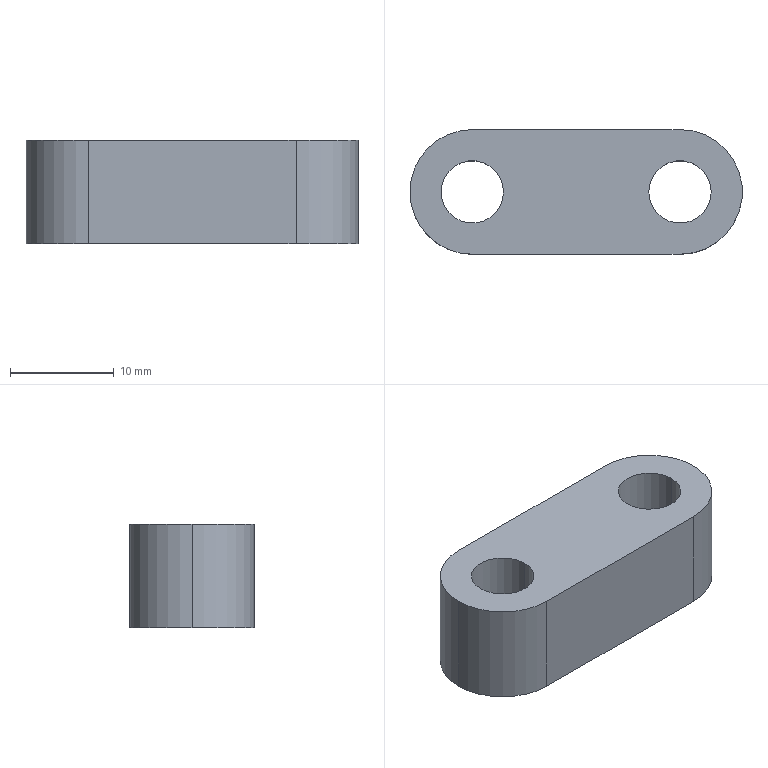Part | SolidWorks | features Extrusion 1 | 1 solid | 11 faces | box 32 x 12 x 10 mm | volume 2965 mm3 | cylinder 7 | plane 4 | commonest cylinder face diameters 6 x4 12 x3
STEP:
#1=CARTESIAN_POINT('',(17.,0.,10.));
#2=VERTEX_POINT('',#1);
#3=CARTESIAN_POINT('',(23.,0.,10.));
#4=VERTEX_POINT('',#3);
#5=CARTESIAN_POINT('',(20.,0.,10.));
#6=DIRECTION('',(0.,0.,1.));
#7=DIRECTION('',(1.,0.,0.));
#8=AXIS2_PLACEMENT_3D('',#5,#6,#7);
#9=CIRCLE('',#8,3.);
#10=EDGE_CURVE('',#2,#4,#9,.T.);
#11=ORIENTED_EDGE('',*,*,#10,.T.);
#12=CARTESIAN_POINT('',(23.,0.,0.));
#13=VERTEX_POINT('',#12);
#14=CARTESIAN_POINT('',(23.,0.,10.));
#15=DIRECTION('',(0.,0.,-1.));
#16=VECTOR('',#15,1000.);
#17=LINE('',#14,#16);
#18=EDGE_CURVE('',#4,#13,#17,.T.);
#19=ORIENTED_EDGE('',*,*,#18,.T.);
#20=CARTESIAN_POINT('',(17.,0.,0.));
#21=VERTEX_POINT('',#20);
#22=CARTESIAN_POINT('',(20.,0.,0.));
#23=DIRECTION('',(0.,0.,1.));
#24=DIRECTION('',(1.,0.,0.));
#25=AXIS2_PLACEMENT_3D('',#22,#23,#24);
#26=CIRCLE('',#25,3.);
#27=EDGE_CURVE('',#21,#13,#26,.T.);
#28=ORIENTED_EDGE('',*,*,#27,.F.);
#29=CARTESIAN_POINT('',(17.,0.,10.));
#30=DIRECTION('',(0.,0.,-1.));
#31=VECTOR('',#30,1000.);
#32=LINE('',#29,#31);
#33=EDGE_CURVE('',#2,#21,#32,.T.);
#34=ORIENTED_EDGE('',*,*,#33,.F.);
#35=EDGE_LOOP('',(#11,#19,#28,#34));
#36=FACE_OUTER_BOUND('',#35,.T.);
#37=CARTESIAN_POINT('',(20.,0.,10.));
#38=DIRECTION('',(0.,0.,-1.));
#39=DIRECTION('',(-1.,0.,0.));
#40=AXIS2_PLACEMENT_3D('',#37,#38,#39);
#41=CYLINDRICAL_SURFACE('',#40,3.);
#42=ADVANCED_FACE('',(#36),#41,.F.);
#43=CARTESIAN_POINT('',(-3.,0.,10.));
#44=VERTEX_POINT('',#43);
#45=CARTESIAN_POINT('',(3.,0.,10.));
#46=VERTEX_POINT('',#45);
#47=CARTESIAN_POINT('',(0.,0.,10.));
#48=DIRECTION('',(0.,0.,1.));
#49=DIRECTION('',(1.,0.,0.));
#50=AXIS2_PLACEMENT_3D('',#47,#48,#49);
#51=CIRCLE('',#50,3.);
#52=EDGE_CURVE('',#44,#46,#51,.T.);
#53=ORIENTED_EDGE('',*,*,#52,.T.);
#54=CARTESIAN_POINT('',(3.,0.,0.));
#55=VERTEX_POINT('',#54);
#56=CARTESIAN_POINT('',(3.,0.,10.));
#57=DIRECTION('',(0.,0.,-1.));
#58=VECTOR('',#57,1000.);
#59=LINE('',#56,#58);
#60=EDGE_CURVE('',#46,#55,#59,.T.);
#61=ORIENTED_EDGE('',*,*,#60,.T.);
#62=CARTESIAN_POINT('',(-3.,0.,0.));
#63=VERTEX_POINT('',#62);
#64=CARTESIAN_POINT('',(0.,0.,0.));
#65=DIRECTION('',(0.,0.,1.));
#66=DIRECTION('',(1.,0.,0.));
#67=AXIS2_PLACEMENT_3D('',#64,#65,#66);
#68=CIRCLE('',#67,3.);
#69=EDGE_CURVE('',#63,#55,#68,.T.);
#70=ORIENTED_EDGE('',*,*,#69,.F.);
#71=CARTESIAN_POINT('',(-3.,0.,10.));
#72=DIRECTION('',(0.,0.,-1.));
#73=VECTOR('',#72,1000.);
#74=LINE('',#71,#73);
#75=EDGE_CURVE('',#44,#63,#74,.T.);
#76=ORIENTED_EDGE('',*,*,#75,.F.);
#77=EDGE_LOOP('',(#53,#61,#70,#76));
#78=FACE_OUTER_BOUND('',#77,.T.);
#79=CARTESIAN_POINT('',(0.,0.,10.));
#80=DIRECTION('',(0.,0.,-1.));
#81=DIRECTION('',(-1.,0.,0.));
#82=AXIS2_PLACEMENT_3D('',#79,#80,#81);
#83=CYLINDRICAL_SURFACE('',#82,3.);
#84=ADVANCED_FACE('',(#78),#83,.F.);
#85=CARTESIAN_POINT('',(-6.,0.,10.));
#86=VERTEX_POINT('',#85);
#87=CARTESIAN_POINT('',(0.,-6.,10.));
#88=VERTEX_POINT('',#87);
#89=CARTESIAN_POINT('',(0.,0.,10.));
#90=DIRECTION('',(0.,0.,1.));
#91=DIRECTION('',(1.,0.,0.));
#92=AXIS2_PLACEMENT_3D('',#89,#90,#91);
#93=CIRCLE('',#92,6.);
#94=EDGE_CURVE('',#86,#88,#93,.T.);
#95=ORIENTED_EDGE('',*,*,#94,.F.);
#96=CARTESIAN_POINT('',(-6.,0.,0.));
#97=VERTEX_POINT('',#96);
#98=CARTESIAN_POINT('',(-6.,0.,10.));
#99=DIRECTION('',(0.,0.,-1.));
#100=VECTOR('',#99,1000.);
#101=LINE('',#98,#100);
#102=EDGE_CURVE('',#86,#97,#101,.T.);
#103=ORIENTED_EDGE('',*,*,#102,.T.);
#104=CARTESIAN_POINT('',(0.,-6.,0.));
#105=VERTEX_POINT('',#104);
#106=CARTESIAN_POINT('',(0.,0.,0.));
#107=DIRECTION('',(0.,0.,1.));
#108=DIRECTION('',(1.,0.,0.));
#109=AXIS2_PLACEMENT_3D('',#106,#107,#108);
#110=CIRCLE('',#109,6.);
#111=EDGE_CURVE('',#97,#105,#110,.T.);
#112=ORIENTED_EDGE('',*,*,#111,.T.);
#113=CARTESIAN_POINT('',(0.,-6.,10.));
#114=DIRECTION('',(0.,0.,-1.));
#115=VECTOR('',#114,1000.);
#116=LINE('',#113,#115);
#117=EDGE_CURVE('',#88,#105,#116,.T.);
#118=ORIENTED_EDGE('',*,*,#117,.F.);
#119=EDGE_LOOP('',(#95,#103,#112,#118));
#120=FACE_OUTER_BOUND('',#119,.T.);
#121=CARTESIAN_POINT('',(0.,0.,10.));
#122=DIRECTION('',(0.,0.,-1.));
#123=DIRECTION('',(-1.,0.,0.));
#124=AXIS2_PLACEMENT_3D('',#121,#122,#123);
#125=CYLINDRICAL_SURFACE('',#124,6.);
#126=ADVANCED_FACE('',(#120),#125,.T.);
#127=ORIENTED_EDGE('',*,*,#52,.F.);
#128=CARTESIAN_POINT('',(0.,0.,10.));
#129=DIRECTION('',(0.,0.,1.));
#130=DIRECTION('',(1.,0.,0.));
#131=AXIS2_PLACEMENT_3D('',#128,#129,#130);
#132=CIRCLE('',#131,3.);
#133=EDGE_CURVE('',#46,#44,#132,.T.);
#134=ORIENTED_EDGE('',*,*,#133,.F.);
#135=EDGE_LOOP('',(#127,#134));
#136=FACE_BOUND('',#135,.T.);
#137=CARTESIAN_POINT('',(0.,6.,10.));
#138=VERTEX_POINT('',#137);
#139=CARTESIAN_POINT('',(0.,0.,10.));
#140=DIRECTION('',(0.,0.,1.));
#141=DIRECTION('',(1.,0.,0.));
#142=AXIS2_PLACEMENT_3D('',#139,#140,#141);
#143=CIRCLE('',#142,6.);
#144=EDGE_CURVE('',#138,#86,#143,.T.);
#145=ORIENTED_EDGE('',*,*,#144,.T.);
#146=ORIENTED_EDGE('',*,*,#94,.T.);
#147=CARTESIAN_POINT('',(20.,-6.,10.));
#148=VERTEX_POINT('',#147);
#149=CARTESIAN_POINT('',(0.,-6.,10.));
#150=DIRECTION('',(1.,0.,0.));
#151=VECTOR('',#150,1000.);
#152=LINE('',#149,#151);
#153=EDGE_CURVE('',#88,#148,#152,.T.);
#154=ORIENTED_EDGE('',*,*,#153,.T.);
#155=CARTESIAN_POINT('',(20.,6.,10.));
#156=VERTEX_POINT('',#155);
#157=CARTESIAN_POINT('',(20.,0.,10.));
#158=DIRECTION('',(0.,0.,1.));
#159=DIRECTION('',(1.,0.,0.));
#160=AXIS2_PLACEMENT_3D('',#157,#158,#159);
#161=CIRCLE('',#160,6.);
#162=EDGE_CURVE('',#148,#156,#161,.T.);
#163=ORIENTED_EDGE('',*,*,#162,.T.);
#164=CARTESIAN_POINT('',(0.,6.,10.));
#165=DIRECTION('',(-1.,0.,0.));
#166=VECTOR('',#165,1000.);
#167=LINE('',#164,#166);
#168=EDGE_CURVE('',#156,#138,#167,.T.);
#169=ORIENTED_EDGE('',*,*,#168,.T.);
#170=EDGE_LOOP('',(#145,#146,#154,#163,#169));
#171=FACE_OUTER_BOUND('',#170,.T.);
#172=ORIENTED_EDGE('',*,*,#10,.F.);
#173=CARTESIAN_POINT('',(20.,0.,10.));
#174=DIRECTION('',(0.,0.,1.));
#175=DIRECTION('',(1.,0.,0.));
#176=AXIS2_PLACEMENT_3D('',#173,#174,#175);
#177=CIRCLE('',#176,3.);
#178=EDGE_CURVE('',#4,#2,#177,.T.);
#179=ORIENTED_EDGE('',*,*,#178,.F.);
#180=EDGE_LOOP('',(#172,#179));
#181=FACE_BOUND('',#180,.T.);
#182=CARTESIAN_POINT('',(0.,0.,10.));
#183=DIRECTION('',(0.,0.,1.));
#184=DIRECTION('',(1.,0.,0.));
#185=AXIS2_PLACEMENT_3D('',#182,#183,#184);
#186=PLANE('',#185);
#187=ADVANCED_FACE('',(#136,#171,#181),#186,.T.);
#188=CARTESIAN_POINT('',(0.,6.,0.));
#189=VERTEX_POINT('',#188);
#190=CARTESIAN_POINT('',(0.,0.,0.));
#191=DIRECTION('',(0.,0.,1.));
#192=DIRECTION('',(1.,0.,0.));
#193=AXIS2_PLACEMENT_3D('',#190,#191,#192);
#194=CIRCLE('',#193,6.);
#195=EDGE_CURVE('',#189,#97,#194,.T.);
#196=ORIENTED_EDGE('',*,*,#195,.F.);
#197=CARTESIAN_POINT('',(20.,6.,0.));
#198=VERTEX_POINT('',#197);
#199=CARTESIAN_POINT('',(0.,6.,0.));
#200=DIRECTION('',(-1.,0.,0.));
#201=VECTOR('',#200,1000.);
#202=LINE('',#199,#201);
#203=EDGE_CURVE('',#198,#189,#202,.T.);
#204=ORIENTED_EDGE('',*,*,#203,.F.);
#205=CARTESIAN_POINT('',(20.,-6.,0.));
#206=VERTEX_POINT('',#205);
#207=CARTESIAN_POINT('',(20.,0.,0.));
#208=DIRECTION('',(0.,0.,1.));
#209=DIRECTION('',(1.,0.,0.));
#210=AXIS2_PLACEMENT_3D('',#207,#208,#209);
#211=CIRCLE('',#210,6.);
#212=EDGE_CURVE('',#206,#198,#211,.T.);
#213=ORIENTED_EDGE('',*,*,#212,.F.);
#214=CARTESIAN_POINT('',(0.,-6.,0.));
#215=DIRECTION('',(1.,0.,0.));
#216=VECTOR('',#215,1000.);
#217=LINE('',#214,#216);
#218=EDGE_CURVE('',#105,#206,#217,.T.);
#219=ORIENTED_EDGE('',*,*,#218,.F.);
#220=ORIENTED_EDGE('',*,*,#111,.F.);
#221=EDGE_LOOP('',(#196,#204,#213,#219,#220));
#222=FACE_OUTER_BOUND('',#221,.T.);
#223=ORIENTED_EDGE('',*,*,#69,.T.);
#224=CARTESIAN_POINT('',(0.,0.,0.));
#225=DIRECTION('',(0.,0.,1.));
#226=DIRECTION('',(1.,0.,0.));
#227=AXIS2_PLACEMENT_3D('',#224,#225,#226);
#228=CIRCLE('',#227,3.);
#229=EDGE_CURVE('',#55,#63,#228,.T.);
#230=ORIENTED_EDGE('',*,*,#229,.T.);
#231=EDGE_LOOP('',(#223,#230));
#232=FACE_BOUND('',#231,.T.);
#233=ORIENTED_EDGE('',*,*,#27,.T.);
#234=CARTESIAN_POINT('',(20.,0.,0.));
#235=DIRECTION('',(0.,0.,1.));
#236=DIRECTION('',(1.,0.,0.));
#237=AXIS2_PLACEMENT_3D('',#234,#235,#236);
#238=CIRCLE('',#237,3.);
#239=EDGE_CURVE('',#13,#21,#238,.T.);
#240=ORIENTED_EDGE('',*,*,#239,.T.);
#241=EDGE_LOOP('',(#233,#240));
#242=FACE_BOUND('',#241,.T.);
#243=CARTESIAN_POINT('',(0.,0.,0.));
#244=DIRECTION('',(0.,0.,1.));
#245=DIRECTION('',(1.,0.,0.));
#246=AXIS2_PLACEMENT_3D('',#243,#244,#245);
#247=PLANE('',#246);
#248=ADVANCED_FACE('',(#222,#232,#242),#247,.F.);
#249=ORIENTED_EDGE('',*,*,#102,.F.);
#250=ORIENTED_EDGE('',*,*,#144,.F.);
#251=CARTESIAN_POINT('',(0.,6.,10.));
#252=DIRECTION('',(0.,0.,-1.));
#253=VECTOR('',#252,1000.);
#254=LINE('',#251,#253);
#255=EDGE_CURVE('',#138,#189,#254,.T.);
#256=ORIENTED_EDGE('',*,*,#255,.T.);
#257=ORIENTED_EDGE('',*,*,#195,.T.);
#258=EDGE_LOOP('',(#249,#250,#256,#257));
#259=FACE_OUTER_BOUND('',#258,.T.);
#260=CARTESIAN_POINT('',(0.,0.,10.));
#261=DIRECTION('',(0.,0.,-1.));
#262=DIRECTION('',(-1.,0.,0.));
#263=AXIS2_PLACEMENT_3D('',#260,#261,#262);
#264=CYLINDRICAL_SURFACE('',#263,6.);
#265=ADVANCED_FACE('',(#259),#264,.T.);
#266=ORIENTED_EDGE('',*,*,#218,.T.);
#267=CARTESIAN_POINT('',(20.,-6.,10.));
#268=DIRECTION('',(0.,0.,-1.));
#269=VECTOR('',#268,1000.);
#270=LINE('',#267,#269);
#271=EDGE_CURVE('',#148,#206,#270,.T.);
#272=ORIENTED_EDGE('',*,*,#271,.F.);
#273=ORIENTED_EDGE('',*,*,#153,.F.);
#274=ORIENTED_EDGE('',*,*,#117,.T.);
#275=EDGE_LOOP('',(#266,#272,#273,#274));
#276=FACE_OUTER_BOUND('',#275,.T.);
#277=CARTESIAN_POINT('',(0.,-6.,10.));
#278=DIRECTION('',(0.,1.,0.));
#279=DIRECTION('',(0.,0.,1.));
#280=AXIS2_PLACEMENT_3D('',#277,#278,#279);
#281=PLANE('',#280);
#282=ADVANCED_FACE('',(#276),#281,.F.);
#283=ORIENTED_EDGE('',*,*,#212,.T.);
#284=CARTESIAN_POINT('',(20.,6.,10.));
#285=DIRECTION('',(0.,0.,-1.));
#286=VECTOR('',#285,1000.);
#287=LINE('',#284,#286);
#288=EDGE_CURVE('',#156,#198,#287,.T.);
#289=ORIENTED_EDGE('',*,*,#288,.F.);
#290=ORIENTED_EDGE('',*,*,#162,.F.);
#291=ORIENTED_EDGE('',*,*,#271,.T.);
#292=EDGE_LOOP('',(#283,#289,#290,#291));
#293=FACE_OUTER_BOUND('',#292,.T.);
#294=CARTESIAN_POINT('',(20.,0.,10.));
#295=DIRECTION('',(0.,0.,-1.));
#296=DIRECTION('',(-1.,0.,0.));
#297=AXIS2_PLACEMENT_3D('',#294,#295,#296);
#298=CYLINDRICAL_SURFACE('',#297,6.);
#299=ADVANCED_FACE('',(#293),#298,.T.);
#300=ORIENTED_EDGE('',*,*,#203,.T.);
#301=ORIENTED_EDGE('',*,*,#255,.F.);
#302=ORIENTED_EDGE('',*,*,#168,.F.);
#303=ORIENTED_EDGE('',*,*,#288,.T.);
#304=EDGE_LOOP('',(#300,#301,#302,#303));
#305=FACE_OUTER_BOUND('',#304,.T.);
#306=CARTESIAN_POINT('',(0.,6.,10.));
#307=DIRECTION('',(0.,-1.,0.));
#308=DIRECTION('',(0.,0.,-1.));
#309=AXIS2_PLACEMENT_3D('',#306,#307,#308);
#310=PLANE('',#309);
#311=ADVANCED_FACE('',(#305),#310,.F.);
#312=ORIENTED_EDGE('',*,*,#60,.F.);
#313=ORIENTED_EDGE('',*,*,#133,.T.);
#314=ORIENTED_EDGE('',*,*,#75,.T.);
#315=ORIENTED_EDGE('',*,*,#229,.F.);
#316=EDGE_LOOP('',(#312,#313,#314,#315));
#317=FACE_OUTER_BOUND('',#316,.T.);
#318=CARTESIAN_POINT('',(0.,0.,10.));
#319=DIRECTION('',(0.,0.,-1.));
#320=DIRECTION('',(-1.,0.,0.));
#321=AXIS2_PLACEMENT_3D('',#318,#319,#320);
#322=CYLINDRICAL_SURFACE('',#321,3.);
#323=ADVANCED_FACE('',(#317),#322,.F.);
#324=ORIENTED_EDGE('',*,*,#18,.F.);
#325=ORIENTED_EDGE('',*,*,#178,.T.);
#326=ORIENTED_EDGE('',*,*,#33,.T.);
#327=ORIENTED_EDGE('',*,*,#239,.F.);
#328=EDGE_LOOP('',(#324,#325,#326,#327));
#329=FACE_OUTER_BOUND('',#328,.T.);
#330=CARTESIAN_POINT('',(20.,0.,10.));
#331=DIRECTION('',(0.,0.,-1.));
#332=DIRECTION('',(-1.,0.,0.));
#333=AXIS2_PLACEMENT_3D('',#330,#331,#332);
#334=CYLINDRICAL_SURFACE('',#333,3.);
#335=ADVANCED_FACE('',(#329),#334,.F.);
#336=CLOSED_SHELL('',(#42,#84,#126,#187,#248,#265,#282,#299,#311,#323,#335));
#337=MANIFOLD_SOLID_BREP('',#336);
#338=CARTESIAN_POINT('',(0.,0.,0.));
#339=DIRECTION('',(0.,0.,1.));
#340=DIRECTION('',(1.,0.,0.));
#341=AXIS2_PLACEMENT_3D('',#338,#339,#340);
#342=(LENGTH_UNIT()NAMED_UNIT(*)SI_UNIT(.MILLI.,.METRE.));
#343=UNCERTAINTY_MEASURE_WITH_UNIT(LENGTH_MEASURE(0.00001),#342,'','');
#344=(NAMED_UNIT(*)PLANE_ANGLE_UNIT()SI_UNIT($,.RADIAN.));
#345=(NAMED_UNIT(*)SI_UNIT($,.STERADIAN.)SOLID_ANGLE_UNIT());
#346=(GEOMETRIC_REPRESENTATION_CONTEXT(3)GLOBAL_UNCERTAINTY_ASSIGNED_CONTEXT((#343))GLOBAL_UNIT_ASSIGNED_CONTEXT((#342,#344,#345))REPRESENTATION_CONTEXT('',''));
#347=ADVANCED_BREP_SHAPE_REPRESENTATION('',(#337,#341),#346);